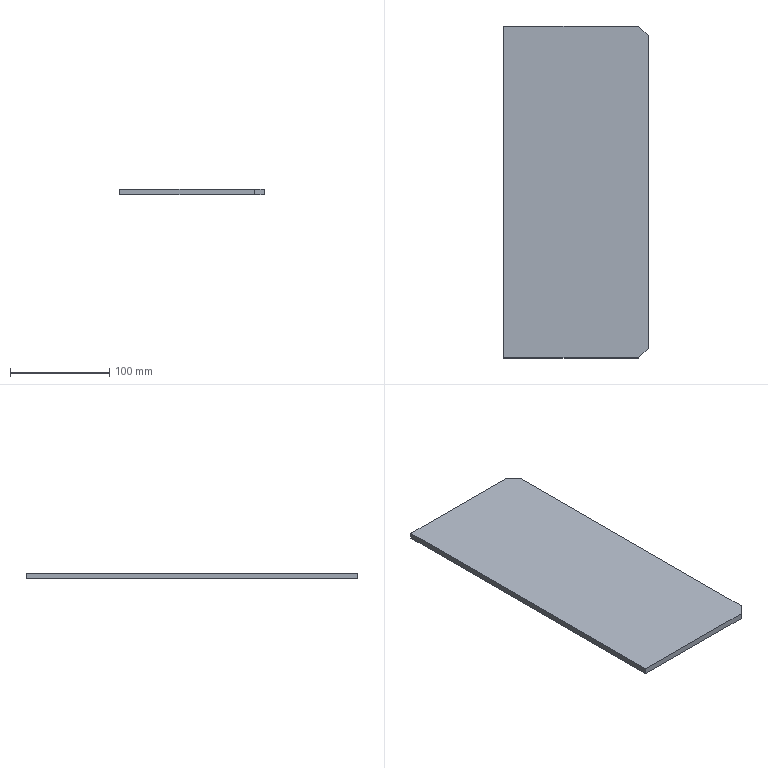Part | STEP file | 02-Rib plate 2 | 1 solid | 8 faces | box 146 x 335 x 6 mm | volume 292860 mm3 | plane 8
STEP:
#1=CARTESIAN_POINT('',(0.,0.,0.));
#2=DIRECTION('',(0.,0.,1.));
#3=DIRECTION('',(1.,0.,0.));
#4=AXIS2_PLACEMENT_3D('',#1,#2,#3);
#5=CARTESIAN_POINT('',(0.,0.,0.));
#6=VERTEX_POINT('',#5);
#7=CARTESIAN_POINT('',(0.,-335.,0.));
#8=VERTEX_POINT('',#7);
#9=CARTESIAN_POINT('',(0.,0.,0.));
#10=DIRECTION('',(0.,-1.,0.));
#11=VECTOR('',#10,1.);
#12=LINE('',#9,#11);
#13=CARTESIAN_POINT('',(0.,0.,6.));
#14=DIRECTION('',(1.,0.,0.));
#15=DIRECTION('',(0.,1.,0.));
#16=AXIS2_PLACEMENT_3D('',#13,#14,#15);
#17=PLANE('',#16);
#18=CARTESIAN_POINT('',(0.,-6.));
#19=DIRECTION('',(-1.,0.));
#20=VECTOR('',#19,1.);
#21=LINE('',#18,#20);
#22=(GEOMETRIC_REPRESENTATION_CONTEXT(2)PARAMETRIC_REPRESENTATION_CONTEXT()REPRESENTATION_CONTEXT('',''));
#23=DEFINITIONAL_REPRESENTATION('',(#21),#22);
#24=PCURVE('',#17,#23);
#25=CARTESIAN_POINT('',(0.,0.,0.));
#26=DIRECTION('',(0.,0.,1.));
#27=DIRECTION('',(1.,0.,0.));
#28=AXIS2_PLACEMENT_3D('',#25,#26,#27);
#29=PLANE('',#28);
#30=CARTESIAN_POINT('',(0.,0.));
#31=DIRECTION('',(0.,-1.));
#32=VECTOR('',#31,1.);
#33=LINE('',#30,#32);
#34=(GEOMETRIC_REPRESENTATION_CONTEXT(2)PARAMETRIC_REPRESENTATION_CONTEXT()REPRESENTATION_CONTEXT('',''));
#35=DEFINITIONAL_REPRESENTATION('',(#33),#34);
#36=PCURVE('',#29,#35);
#37=SURFACE_CURVE('',#12,(#24,#36),.PCURVE_S1.);
#38=EDGE_CURVE('',#6,#8,#37,.T.);
#39=ORIENTED_EDGE('',*,*,#38,.T.);
#40=CARTESIAN_POINT('',(0.,-335.,6.));
#41=VERTEX_POINT('',#40);
#42=CARTESIAN_POINT('',(0.,-335.,6.));
#43=DIRECTION('',(0.,0.,-1.));
#44=VECTOR('',#43,1.);
#45=LINE('',#42,#44);
#46=CARTESIAN_POINT('',(-335.,0.));
#47=DIRECTION('',(0.,-1.));
#48=VECTOR('',#47,1.);
#49=LINE('',#46,#48);
#50=(GEOMETRIC_REPRESENTATION_CONTEXT(2)PARAMETRIC_REPRESENTATION_CONTEXT()REPRESENTATION_CONTEXT('',''));
#51=DEFINITIONAL_REPRESENTATION('',(#49),#50);
#52=PCURVE('',#17,#51);
#53=CARTESIAN_POINT('',(0.,-335.,6.));
#54=DIRECTION('',(0.,1.,0.));
#55=DIRECTION('',(0.,0.,1.));
#56=AXIS2_PLACEMENT_3D('',#53,#54,#55);
#57=PLANE('',#56);
#58=CARTESIAN_POINT('',(0.,0.));
#59=DIRECTION('',(-1.,0.));
#60=VECTOR('',#59,1.);
#61=LINE('',#58,#60);
#62=(GEOMETRIC_REPRESENTATION_CONTEXT(2)PARAMETRIC_REPRESENTATION_CONTEXT()REPRESENTATION_CONTEXT('',''));
#63=DEFINITIONAL_REPRESENTATION('',(#61),#62);
#64=PCURVE('',#57,#63);
#65=SURFACE_CURVE('',#45,(#52,#64),.PCURVE_S1.);
#66=EDGE_CURVE('',#41,#8,#65,.T.);
#67=ORIENTED_EDGE('',*,*,#66,.F.);
#68=CARTESIAN_POINT('',(0.,0.,6.));
#69=VERTEX_POINT('',#68);
#70=CARTESIAN_POINT('',(0.,0.,6.));
#71=DIRECTION('',(0.,-1.,0.));
#72=VECTOR('',#71,1.);
#73=LINE('',#70,#72);
#74=CARTESIAN_POINT('',(0.,0.));
#75=DIRECTION('',(-1.,0.));
#76=VECTOR('',#75,1.);
#77=LINE('',#74,#76);
#78=(GEOMETRIC_REPRESENTATION_CONTEXT(2)PARAMETRIC_REPRESENTATION_CONTEXT()REPRESENTATION_CONTEXT('',''));
#79=DEFINITIONAL_REPRESENTATION('',(#77),#78);
#80=PCURVE('',#17,#79);
#81=CARTESIAN_POINT('',(0.,0.,6.));
#82=DIRECTION('',(0.,0.,1.));
#83=DIRECTION('',(1.,0.,0.));
#84=AXIS2_PLACEMENT_3D('',#81,#82,#83);
#85=PLANE('',#84);
#86=CARTESIAN_POINT('',(0.,0.));
#87=DIRECTION('',(0.,-1.));
#88=VECTOR('',#87,1.);
#89=LINE('',#86,#88);
#90=(GEOMETRIC_REPRESENTATION_CONTEXT(2)PARAMETRIC_REPRESENTATION_CONTEXT()REPRESENTATION_CONTEXT('',''));
#91=DEFINITIONAL_REPRESENTATION('',(#89),#90);
#92=PCURVE('',#85,#91);
#93=SURFACE_CURVE('',#73,(#80,#92),.PCURVE_S1.);
#94=EDGE_CURVE('',#69,#41,#93,.T.);
#95=ORIENTED_EDGE('',*,*,#94,.F.);
#96=CARTESIAN_POINT('',(0.,0.,6.));
#97=DIRECTION('',(0.,0.,-1.));
#98=VECTOR('',#97,1.);
#99=LINE('',#96,#98);
#100=CARTESIAN_POINT('',(0.,0.));
#101=DIRECTION('',(0.,-1.));
#102=VECTOR('',#101,1.);
#103=LINE('',#100,#102);
#104=(GEOMETRIC_REPRESENTATION_CONTEXT(2)PARAMETRIC_REPRESENTATION_CONTEXT()REPRESENTATION_CONTEXT('',''));
#105=DEFINITIONAL_REPRESENTATION('',(#103),#104);
#106=PCURVE('',#17,#105);
#107=CARTESIAN_POINT('',(0.,0.,6.));
#108=DIRECTION('',(0.,-1.,0.));
#109=DIRECTION('',(0.,0.,-1.));
#110=AXIS2_PLACEMENT_3D('',#107,#108,#109);
#111=PLANE('',#110);
#112=CARTESIAN_POINT('',(0.,0.));
#113=DIRECTION('',(1.,0.));
#114=VECTOR('',#113,1.);
#115=LINE('',#112,#114);
#116=(GEOMETRIC_REPRESENTATION_CONTEXT(2)PARAMETRIC_REPRESENTATION_CONTEXT()REPRESENTATION_CONTEXT('',''));
#117=DEFINITIONAL_REPRESENTATION('',(#115),#116);
#118=PCURVE('',#111,#117);
#119=SURFACE_CURVE('',#99,(#106,#118),.PCURVE_S1.);
#120=EDGE_CURVE('',#69,#6,#119,.T.);
#121=ORIENTED_EDGE('',*,*,#120,.T.);
#122=EDGE_LOOP('',(#39,#67,#95,#121));
#123=FACE_BOUND('',#122,.T.);
#124=ADVANCED_FACE('',(#123),#17,.F.);
#125=CARTESIAN_POINT('',(136.,-335.,0.));
#126=VERTEX_POINT('',#125);
#127=CARTESIAN_POINT('',(0.,-335.,0.));
#128=DIRECTION('',(1.,0.,0.));
#129=VECTOR('',#128,1.);
#130=LINE('',#127,#129);
#131=CARTESIAN_POINT('',(-6.,0.));
#132=DIRECTION('',(0.,1.));
#133=VECTOR('',#132,1.);
#134=LINE('',#131,#133);
#135=(GEOMETRIC_REPRESENTATION_CONTEXT(2)PARAMETRIC_REPRESENTATION_CONTEXT()REPRESENTATION_CONTEXT('',''));
#136=DEFINITIONAL_REPRESENTATION('',(#134),#135);
#137=PCURVE('',#57,#136);
#138=CARTESIAN_POINT('',(0.,-335.));
#139=DIRECTION('',(1.,0.));
#140=VECTOR('',#139,1.);
#141=LINE('',#138,#140);
#142=(GEOMETRIC_REPRESENTATION_CONTEXT(2)PARAMETRIC_REPRESENTATION_CONTEXT()REPRESENTATION_CONTEXT('',''));
#143=DEFINITIONAL_REPRESENTATION('',(#141),#142);
#144=PCURVE('',#29,#143);
#145=SURFACE_CURVE('',#130,(#137,#144),.PCURVE_S1.);
#146=EDGE_CURVE('',#8,#126,#145,.T.);
#147=ORIENTED_EDGE('',*,*,#146,.T.);
#148=CARTESIAN_POINT('',(136.,-335.,6.));
#149=VERTEX_POINT('',#148);
#150=CARTESIAN_POINT('',(136.,-335.,6.));
#151=DIRECTION('',(0.,0.,-1.));
#152=VECTOR('',#151,1.);
#153=LINE('',#150,#152);
#154=CARTESIAN_POINT('',(0.,136.));
#155=DIRECTION('',(-1.,0.));
#156=VECTOR('',#155,1.);
#157=LINE('',#154,#156);
#158=(GEOMETRIC_REPRESENTATION_CONTEXT(2)PARAMETRIC_REPRESENTATION_CONTEXT()REPRESENTATION_CONTEXT('',''));
#159=DEFINITIONAL_REPRESENTATION('',(#157),#158);
#160=PCURVE('',#57,#159);
#161=CARTESIAN_POINT('',(146.,-325.,6.));
#162=DIRECTION('',(-0.7071,0.7071,0.));
#163=DIRECTION('',(-0.7071,-0.7071,0.));
#164=AXIS2_PLACEMENT_3D('',#161,#162,#163);
#165=PLANE('',#164);
#166=CARTESIAN_POINT('',(14.142,0.));
#167=DIRECTION('',(0.,-1.));
#168=VECTOR('',#167,1.);
#169=LINE('',#166,#168);
#170=(GEOMETRIC_REPRESENTATION_CONTEXT(2)PARAMETRIC_REPRESENTATION_CONTEXT()REPRESENTATION_CONTEXT('',''));
#171=DEFINITIONAL_REPRESENTATION('',(#169),#170);
#172=PCURVE('',#165,#171);
#173=SURFACE_CURVE('',#153,(#160,#172),.PCURVE_S1.);
#174=EDGE_CURVE('',#149,#126,#173,.T.);
#175=ORIENTED_EDGE('',*,*,#174,.F.);
#176=CARTESIAN_POINT('',(0.,-335.,6.));
#177=DIRECTION('',(1.,0.,0.));
#178=VECTOR('',#177,1.);
#179=LINE('',#176,#178);
#180=CARTESIAN_POINT('',(0.,0.));
#181=DIRECTION('',(0.,1.));
#182=VECTOR('',#181,1.);
#183=LINE('',#180,#182);
#184=(GEOMETRIC_REPRESENTATION_CONTEXT(2)PARAMETRIC_REPRESENTATION_CONTEXT()REPRESENTATION_CONTEXT('',''));
#185=DEFINITIONAL_REPRESENTATION('',(#183),#184);
#186=PCURVE('',#57,#185);
#187=CARTESIAN_POINT('',(0.,-335.));
#188=DIRECTION('',(1.,0.));
#189=VECTOR('',#188,1.);
#190=LINE('',#187,#189);
#191=(GEOMETRIC_REPRESENTATION_CONTEXT(2)PARAMETRIC_REPRESENTATION_CONTEXT()REPRESENTATION_CONTEXT('',''));
#192=DEFINITIONAL_REPRESENTATION('',(#190),#191);
#193=PCURVE('',#85,#192);
#194=SURFACE_CURVE('',#179,(#186,#193),.PCURVE_S1.);
#195=EDGE_CURVE('',#41,#149,#194,.T.);
#196=ORIENTED_EDGE('',*,*,#195,.F.);
#197=ORIENTED_EDGE('',*,*,#66,.T.);
#198=EDGE_LOOP('',(#147,#175,#196,#197));
#199=FACE_BOUND('',#198,.T.);
#200=ADVANCED_FACE('',(#199),#57,.F.);
#201=CARTESIAN_POINT('',(146.,-325.,0.));
#202=VERTEX_POINT('',#201);
#203=CARTESIAN_POINT('',(146.,-325.,0.));
#204=DIRECTION('',(0.7071,0.7071,0.));
#205=VECTOR('',#204,1.);
#206=LINE('',#203,#205);
#207=CARTESIAN_POINT('',(0.,-6.));
#208=DIRECTION('',(-1.,0.));
#209=VECTOR('',#208,1.);
#210=LINE('',#207,#209);
#211=(GEOMETRIC_REPRESENTATION_CONTEXT(2)PARAMETRIC_REPRESENTATION_CONTEXT()REPRESENTATION_CONTEXT('',''));
#212=DEFINITIONAL_REPRESENTATION('',(#210),#211);
#213=PCURVE('',#165,#212);
#214=CARTESIAN_POINT('',(146.,-325.));
#215=DIRECTION('',(0.7071,0.7071));
#216=VECTOR('',#215,1.);
#217=LINE('',#214,#216);
#218=(GEOMETRIC_REPRESENTATION_CONTEXT(2)PARAMETRIC_REPRESENTATION_CONTEXT()REPRESENTATION_CONTEXT('',''));
#219=DEFINITIONAL_REPRESENTATION('',(#217),#218);
#220=PCURVE('',#29,#219);
#221=SURFACE_CURVE('',#206,(#213,#220),.PCURVE_S1.);
#222=EDGE_CURVE('',#126,#202,#221,.T.);
#223=ORIENTED_EDGE('',*,*,#222,.T.);
#224=CARTESIAN_POINT('',(146.,-325.,6.));
#225=VERTEX_POINT('',#224);
#226=CARTESIAN_POINT('',(146.,-325.,6.));
#227=DIRECTION('',(0.,0.,-1.));
#228=VECTOR('',#227,1.);
#229=LINE('',#226,#228);
#230=CARTESIAN_POINT('',(0.,0.));
#231=DIRECTION('',(0.,-1.));
#232=VECTOR('',#231,1.);
#233=LINE('',#230,#232);
#234=(GEOMETRIC_REPRESENTATION_CONTEXT(2)PARAMETRIC_REPRESENTATION_CONTEXT()REPRESENTATION_CONTEXT('',''));
#235=DEFINITIONAL_REPRESENTATION('',(#233),#234);
#236=PCURVE('',#165,#235);
#237=CARTESIAN_POINT('',(146.,-10.,6.));
#238=DIRECTION('',(-1.,0.,0.));
#239=DIRECTION('',(0.,-1.,0.));
#240=AXIS2_PLACEMENT_3D('',#237,#238,#239);
#241=PLANE('',#240);
#242=CARTESIAN_POINT('',(315.,0.));
#243=DIRECTION('',(0.,-1.));
#244=VECTOR('',#243,1.);
#245=LINE('',#242,#244);
#246=(GEOMETRIC_REPRESENTATION_CONTEXT(2)PARAMETRIC_REPRESENTATION_CONTEXT()REPRESENTATION_CONTEXT('',''));
#247=DEFINITIONAL_REPRESENTATION('',(#245),#246);
#248=PCURVE('',#241,#247);
#249=SURFACE_CURVE('',#229,(#236,#248),.PCURVE_S1.);
#250=EDGE_CURVE('',#225,#202,#249,.T.);
#251=ORIENTED_EDGE('',*,*,#250,.F.);
#252=CARTESIAN_POINT('',(146.,-325.,6.));
#253=DIRECTION('',(0.7071,0.7071,0.));
#254=VECTOR('',#253,1.);
#255=LINE('',#252,#254);
#256=CARTESIAN_POINT('',(0.,0.));
#257=DIRECTION('',(-1.,0.));
#258=VECTOR('',#257,1.);
#259=LINE('',#256,#258);
#260=(GEOMETRIC_REPRESENTATION_CONTEXT(2)PARAMETRIC_REPRESENTATION_CONTEXT()REPRESENTATION_CONTEXT('',''));
#261=DEFINITIONAL_REPRESENTATION('',(#259),#260);
#262=PCURVE('',#165,#261);
#263=CARTESIAN_POINT('',(146.,-325.));
#264=DIRECTION('',(0.7071,0.7071));
#265=VECTOR('',#264,1.);
#266=LINE('',#263,#265);
#267=(GEOMETRIC_REPRESENTATION_CONTEXT(2)PARAMETRIC_REPRESENTATION_CONTEXT()REPRESENTATION_CONTEXT('',''));
#268=DEFINITIONAL_REPRESENTATION('',(#266),#267);
#269=PCURVE('',#85,#268);
#270=SURFACE_CURVE('',#255,(#262,#269),.PCURVE_S1.);
#271=EDGE_CURVE('',#149,#225,#270,.T.);
#272=ORIENTED_EDGE('',*,*,#271,.F.);
#273=ORIENTED_EDGE('',*,*,#174,.T.);
#274=EDGE_LOOP('',(#223,#251,#272,#273));
#275=FACE_BOUND('',#274,.T.);
#276=ADVANCED_FACE('',(#275),#165,.F.);
#277=CARTESIAN_POINT('',(146.,-10.,0.));
#278=VERTEX_POINT('',#277);
#279=CARTESIAN_POINT('',(146.,-10.,0.));
#280=DIRECTION('',(0.,1.,0.));
#281=VECTOR('',#280,1.);
#282=LINE('',#279,#281);
#283=CARTESIAN_POINT('',(0.,-6.));
#284=DIRECTION('',(-1.,0.));
#285=VECTOR('',#284,1.);
#286=LINE('',#283,#285);
#287=(GEOMETRIC_REPRESENTATION_CONTEXT(2)PARAMETRIC_REPRESENTATION_CONTEXT()REPRESENTATION_CONTEXT('',''));
#288=DEFINITIONAL_REPRESENTATION('',(#286),#287);
#289=PCURVE('',#241,#288);
#290=CARTESIAN_POINT('',(146.,-10.));
#291=DIRECTION('',(0.,1.));
#292=VECTOR('',#291,1.);
#293=LINE('',#290,#292);
#294=(GEOMETRIC_REPRESENTATION_CONTEXT(2)PARAMETRIC_REPRESENTATION_CONTEXT()REPRESENTATION_CONTEXT('',''));
#295=DEFINITIONAL_REPRESENTATION('',(#293),#294);
#296=PCURVE('',#29,#295);
#297=SURFACE_CURVE('',#282,(#289,#296),.PCURVE_S1.);
#298=EDGE_CURVE('',#202,#278,#297,.T.);
#299=ORIENTED_EDGE('',*,*,#298,.T.);
#300=CARTESIAN_POINT('',(146.,-10.,6.));
#301=VERTEX_POINT('',#300);
#302=CARTESIAN_POINT('',(146.,-10.,6.));
#303=DIRECTION('',(0.,0.,-1.));
#304=VECTOR('',#303,1.);
#305=LINE('',#302,#304);
#306=CARTESIAN_POINT('',(0.,0.));
#307=DIRECTION('',(0.,-1.));
#308=VECTOR('',#307,1.);
#309=LINE('',#306,#308);
#310=(GEOMETRIC_REPRESENTATION_CONTEXT(2)PARAMETRIC_REPRESENTATION_CONTEXT()REPRESENTATION_CONTEXT('',''));
#311=DEFINITIONAL_REPRESENTATION('',(#309),#310);
#312=PCURVE('',#241,#311);
#313=CARTESIAN_POINT('',(136.,0.,6.));
#314=DIRECTION('',(-0.7071,-0.7071,0.));
#315=DIRECTION('',(0.7071,-0.7071,0.));
#316=AXIS2_PLACEMENT_3D('',#313,#314,#315);
#317=PLANE('',#316);
#318=CARTESIAN_POINT('',(14.142,0.));
#319=DIRECTION('',(0.,-1.));
#320=VECTOR('',#319,1.);
#321=LINE('',#318,#320);
#322=(GEOMETRIC_REPRESENTATION_CONTEXT(2)PARAMETRIC_REPRESENTATION_CONTEXT()REPRESENTATION_CONTEXT('',''));
#323=DEFINITIONAL_REPRESENTATION('',(#321),#322);
#324=PCURVE('',#317,#323);
#325=SURFACE_CURVE('',#305,(#312,#324),.PCURVE_S1.);
#326=EDGE_CURVE('',#301,#278,#325,.T.);
#327=ORIENTED_EDGE('',*,*,#326,.F.);
#328=CARTESIAN_POINT('',(146.,-10.,6.));
#329=DIRECTION('',(0.,1.,0.));
#330=VECTOR('',#329,1.);
#331=LINE('',#328,#330);
#332=CARTESIAN_POINT('',(0.,0.));
#333=DIRECTION('',(-1.,0.));
#334=VECTOR('',#333,1.);
#335=LINE('',#332,#334);
#336=(GEOMETRIC_REPRESENTATION_CONTEXT(2)PARAMETRIC_REPRESENTATION_CONTEXT()REPRESENTATION_CONTEXT('',''));
#337=DEFINITIONAL_REPRESENTATION('',(#335),#336);
#338=PCURVE('',#241,#337);
#339=CARTESIAN_POINT('',(146.,-10.));
#340=DIRECTION('',(0.,1.));
#341=VECTOR('',#340,1.);
#342=LINE('',#339,#341);
#343=(GEOMETRIC_REPRESENTATION_CONTEXT(2)PARAMETRIC_REPRESENTATION_CONTEXT()REPRESENTATION_CONTEXT('',''));
#344=DEFINITIONAL_REPRESENTATION('',(#342),#343);
#345=PCURVE('',#85,#344);
#346=SURFACE_CURVE('',#331,(#338,#345),.PCURVE_S1.);
#347=EDGE_CURVE('',#225,#301,#346,.T.);
#348=ORIENTED_EDGE('',*,*,#347,.F.);
#349=ORIENTED_EDGE('',*,*,#250,.T.);
#350=EDGE_LOOP('',(#299,#327,#348,#349));
#351=FACE_BOUND('',#350,.T.);
#352=ADVANCED_FACE('',(#351),#241,.F.);
#353=CARTESIAN_POINT('',(136.,0.,0.));
#354=VERTEX_POINT('',#353);
#355=CARTESIAN_POINT('',(136.,0.,0.));
#356=DIRECTION('',(-0.7071,0.7071,0.));
#357=VECTOR('',#356,1.);
#358=LINE('',#355,#357);
#359=CARTESIAN_POINT('',(0.,-6.));
#360=DIRECTION('',(-1.,0.));
#361=VECTOR('',#360,1.);
#362=LINE('',#359,#361);
#363=(GEOMETRIC_REPRESENTATION_CONTEXT(2)PARAMETRIC_REPRESENTATION_CONTEXT()REPRESENTATION_CONTEXT('',''));
#364=DEFINITIONAL_REPRESENTATION('',(#362),#363);
#365=PCURVE('',#317,#364);
#366=CARTESIAN_POINT('',(136.,0.));
#367=DIRECTION('',(-0.7071,0.7071));
#368=VECTOR('',#367,1.);
#369=LINE('',#366,#368);
#370=(GEOMETRIC_REPRESENTATION_CONTEXT(2)PARAMETRIC_REPRESENTATION_CONTEXT()REPRESENTATION_CONTEXT('',''));
#371=DEFINITIONAL_REPRESENTATION('',(#369),#370);
#372=PCURVE('',#29,#371);
#373=SURFACE_CURVE('',#358,(#365,#372),.PCURVE_S1.);
#374=EDGE_CURVE('',#278,#354,#373,.T.);
#375=ORIENTED_EDGE('',*,*,#374,.T.);
#376=CARTESIAN_POINT('',(136.,0.,6.));
#377=VERTEX_POINT('',#376);
#378=CARTESIAN_POINT('',(136.,0.,6.));
#379=DIRECTION('',(0.,0.,-1.));
#380=VECTOR('',#379,1.);
#381=LINE('',#378,#380);
#382=CARTESIAN_POINT('',(0.,0.));
#383=DIRECTION('',(0.,-1.));
#384=VECTOR('',#383,1.);
#385=LINE('',#382,#384);
#386=(GEOMETRIC_REPRESENTATION_CONTEXT(2)PARAMETRIC_REPRESENTATION_CONTEXT()REPRESENTATION_CONTEXT('',''));
#387=DEFINITIONAL_REPRESENTATION('',(#385),#386);
#388=PCURVE('',#317,#387);
#389=CARTESIAN_POINT('',(0.,136.));
#390=DIRECTION('',(1.,0.));
#391=VECTOR('',#390,1.);
#392=LINE('',#389,#391);
#393=(GEOMETRIC_REPRESENTATION_CONTEXT(2)PARAMETRIC_REPRESENTATION_CONTEXT()REPRESENTATION_CONTEXT('',''));
#394=DEFINITIONAL_REPRESENTATION('',(#392),#393);
#395=PCURVE('',#111,#394);
#396=SURFACE_CURVE('',#381,(#388,#395),.PCURVE_S1.);
#397=EDGE_CURVE('',#377,#354,#396,.T.);
#398=ORIENTED_EDGE('',*,*,#397,.F.);
#399=CARTESIAN_POINT('',(136.,0.,6.));
#400=DIRECTION('',(-0.7071,0.7071,0.));
#401=VECTOR('',#400,1.);
#402=LINE('',#399,#401);
#403=CARTESIAN_POINT('',(0.,0.));
#404=DIRECTION('',(-1.,0.));
#405=VECTOR('',#404,1.);
#406=LINE('',#403,#405);
#407=(GEOMETRIC_REPRESENTATION_CONTEXT(2)PARAMETRIC_REPRESENTATION_CONTEXT()REPRESENTATION_CONTEXT('',''));
#408=DEFINITIONAL_REPRESENTATION('',(#406),#407);
#409=PCURVE('',#317,#408);
#410=CARTESIAN_POINT('',(136.,0.));
#411=DIRECTION('',(-0.7071,0.7071));
#412=VECTOR('',#411,1.);
#413=LINE('',#410,#412);
#414=(GEOMETRIC_REPRESENTATION_CONTEXT(2)PARAMETRIC_REPRESENTATION_CONTEXT()REPRESENTATION_CONTEXT('',''));
#415=DEFINITIONAL_REPRESENTATION('',(#413),#414);
#416=PCURVE('',#85,#415);
#417=SURFACE_CURVE('',#402,(#409,#416),.PCURVE_S1.);
#418=EDGE_CURVE('',#301,#377,#417,.T.);
#419=ORIENTED_EDGE('',*,*,#418,.F.);
#420=ORIENTED_EDGE('',*,*,#326,.T.);
#421=EDGE_LOOP('',(#375,#398,#419,#420));
#422=FACE_BOUND('',#421,.T.);
#423=ADVANCED_FACE('',(#422),#317,.F.);
#424=CARTESIAN_POINT('',(0.,0.,0.));
#425=DIRECTION('',(-1.,0.,0.));
#426=VECTOR('',#425,1.);
#427=LINE('',#424,#426);
#428=CARTESIAN_POINT('',(6.,0.));
#429=DIRECTION('',(0.,-1.));
#430=VECTOR('',#429,1.);
#431=LINE('',#428,#430);
#432=(GEOMETRIC_REPRESENTATION_CONTEXT(2)PARAMETRIC_REPRESENTATION_CONTEXT()REPRESENTATION_CONTEXT('',''));
#433=DEFINITIONAL_REPRESENTATION('',(#431),#432);
#434=PCURVE('',#111,#433);
#435=CARTESIAN_POINT('',(0.,0.));
#436=DIRECTION('',(-1.,0.));
#437=VECTOR('',#436,1.);
#438=LINE('',#435,#437);
#439=(GEOMETRIC_REPRESENTATION_CONTEXT(2)PARAMETRIC_REPRESENTATION_CONTEXT()REPRESENTATION_CONTEXT('',''));
#440=DEFINITIONAL_REPRESENTATION('',(#438),#439);
#441=PCURVE('',#29,#440);
#442=SURFACE_CURVE('',#427,(#434,#441),.PCURVE_S1.);
#443=EDGE_CURVE('',#354,#6,#442,.T.);
#444=ORIENTED_EDGE('',*,*,#443,.T.);
#445=ORIENTED_EDGE('',*,*,#120,.F.);
#446=CARTESIAN_POINT('',(0.,0.,6.));
#447=DIRECTION('',(-1.,0.,0.));
#448=VECTOR('',#447,1.);
#449=LINE('',#446,#448);
#450=CARTESIAN_POINT('',(0.,0.));
#451=DIRECTION('',(0.,-1.));
#452=VECTOR('',#451,1.);
#453=LINE('',#450,#452);
#454=(GEOMETRIC_REPRESENTATION_CONTEXT(2)PARAMETRIC_REPRESENTATION_CONTEXT()REPRESENTATION_CONTEXT('',''));
#455=DEFINITIONAL_REPRESENTATION('',(#453),#454);
#456=PCURVE('',#111,#455);
#457=CARTESIAN_POINT('',(0.,0.));
#458=DIRECTION('',(-1.,0.));
#459=VECTOR('',#458,1.);
#460=LINE('',#457,#459);
#461=(GEOMETRIC_REPRESENTATION_CONTEXT(2)PARAMETRIC_REPRESENTATION_CONTEXT()REPRESENTATION_CONTEXT('',''));
#462=DEFINITIONAL_REPRESENTATION('',(#460),#461);
#463=PCURVE('',#85,#462);
#464=SURFACE_CURVE('',#449,(#456,#463),.PCURVE_S1.);
#465=EDGE_CURVE('',#377,#69,#464,.T.);
#466=ORIENTED_EDGE('',*,*,#465,.F.);
#467=ORIENTED_EDGE('',*,*,#397,.T.);
#468=EDGE_LOOP('',(#444,#445,#466,#467));
#469=FACE_BOUND('',#468,.T.);
#470=ADVANCED_FACE('',(#469),#111,.F.);
#471=ORIENTED_EDGE('',*,*,#94,.T.);
#472=ORIENTED_EDGE('',*,*,#195,.T.);
#473=ORIENTED_EDGE('',*,*,#271,.T.);
#474=ORIENTED_EDGE('',*,*,#347,.T.);
#475=ORIENTED_EDGE('',*,*,#418,.T.);
#476=ORIENTED_EDGE('',*,*,#465,.T.);
#477=EDGE_LOOP('',(#471,#472,#473,#474,#475,#476));
#478=FACE_BOUND('',#477,.T.);
#479=ADVANCED_FACE('',(#478),#85,.T.);
#480=ORIENTED_EDGE('',*,*,#38,.F.);
#481=ORIENTED_EDGE('',*,*,#443,.F.);
#482=ORIENTED_EDGE('',*,*,#374,.F.);
#483=ORIENTED_EDGE('',*,*,#298,.F.);
#484=ORIENTED_EDGE('',*,*,#222,.F.);
#485=ORIENTED_EDGE('',*,*,#146,.F.);
#486=EDGE_LOOP('',(#480,#481,#482,#483,#484,#485));
#487=FACE_BOUND('',#486,.T.);
#488=ADVANCED_FACE('',(#487),#29,.F.);
#489=CLOSED_SHELL('',(#124,#200,#276,#352,#423,#470,#479,#488));
#490=MANIFOLD_SOLID_BREP('',#489);
#491=(LENGTH_UNIT()NAMED_UNIT(*)SI_UNIT(.MILLI.,.METRE.));
#492=UNCERTAINTY_MEASURE_WITH_UNIT(LENGTH_MEASURE(0.0000001),#491,'','');
#493=(NAMED_UNIT(*)PLANE_ANGLE_UNIT()SI_UNIT($,.RADIAN.));
#494=(NAMED_UNIT(*)SI_UNIT($,.STERADIAN.)SOLID_ANGLE_UNIT());
#495=(GEOMETRIC_REPRESENTATION_CONTEXT(3)GLOBAL_UNCERTAINTY_ASSIGNED_CONTEXT((#492))GLOBAL_UNIT_ASSIGNED_CONTEXT((#491,#493,#494))REPRESENTATION_CONTEXT('',''));
#496=ADVANCED_BREP_SHAPE_REPRESENTATION('',(#4,#490),#495);